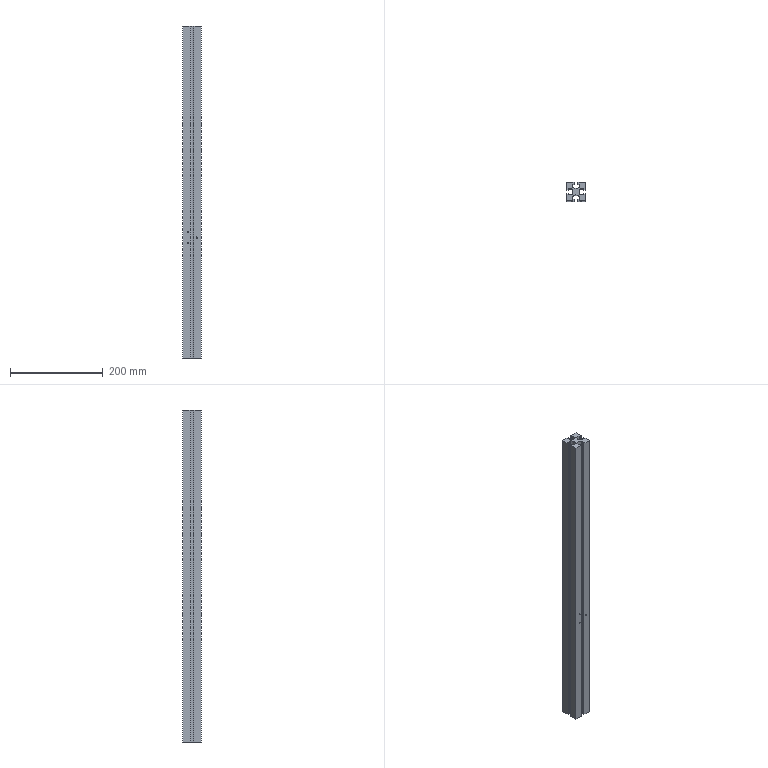Part | NX | 1 solid | 44 faces | box 40 x 40 x 716 mm | volume 715892 mm3 | plane 34 | cylinder 10 | commonest cylinder face diameters 2.5 x6 19.333 x2 19.4 x2
STEP:
#1=CARTESIAN_POINT('',(-125.,655.75,0.));
#2=VERTEX_POINT('',#1);
#3=CARTESIAN_POINT('',(-121.5,655.75,0.));
#4=VERTEX_POINT('',#3);
#5=CARTESIAN_POINT('',(-125.,655.75,0.));
#6=DIRECTION('',(1.,0.,0.));
#7=VECTOR('',#6,1000.);
#8=LINE('',#5,#7);
#9=EDGE_CURVE('',#2,#4,#8,.T.);
#10=ORIENTED_EDGE('',*,*,#9,.T.);
#11=CARTESIAN_POINT('',(-121.5,655.75,-716.));
#12=VERTEX_POINT('',#11);
#13=CARTESIAN_POINT('',(-121.5,655.75,-716.));
#14=DIRECTION('',(0.,0.,1.));
#15=VECTOR('',#14,1000.);
#16=LINE('',#13,#15);
#17=EDGE_CURVE('',#12,#4,#16,.T.);
#18=ORIENTED_EDGE('',*,*,#17,.F.);
#19=CARTESIAN_POINT('',(-125.,655.75,-716.));
#20=VERTEX_POINT('',#19);
#21=CARTESIAN_POINT('',(-125.,655.75,-716.));
#22=DIRECTION('',(1.,0.,0.));
#23=VECTOR('',#22,1000.);
#24=LINE('',#21,#23);
#25=EDGE_CURVE('',#20,#12,#24,.T.);
#26=ORIENTED_EDGE('',*,*,#25,.F.);
#27=CARTESIAN_POINT('',(-125.,655.75,-716.));
#28=DIRECTION('',(0.,0.,1.));
#29=VECTOR('',#28,1000.);
#30=LINE('',#27,#29);
#31=EDGE_CURVE('',#20,#2,#30,.T.);
#32=ORIENTED_EDGE('',*,*,#31,.T.);
#33=EDGE_LOOP('',(#10,#18,#26,#32));
#34=FACE_BOUND('',#33,.T.);
#35=CARTESIAN_POINT('',(-125.,655.75,-716.));
#36=DIRECTION('',(0.,-1.,0.));
#37=DIRECTION('',(0.,0.,-1.));
#38=AXIS2_PLACEMENT_3D('',#35,#36,#37);
#39=PLANE('',#38);
#40=ADVANCED_FACE('',(#34),#39,.F.);
#41=CARTESIAN_POINT('',(-121.5,653.,0.));
#42=VERTEX_POINT('',#41);
#43=CARTESIAN_POINT('',(-121.5,655.75,0.));
#44=DIRECTION('',(0.,-1.,0.));
#45=VECTOR('',#44,1000.);
#46=LINE('',#43,#45);
#47=EDGE_CURVE('',#4,#42,#46,.T.);
#48=ORIENTED_EDGE('',*,*,#47,.T.);
#49=CARTESIAN_POINT('',(-121.5,653.,-716.));
#50=VERTEX_POINT('',#49);
#51=CARTESIAN_POINT('',(-121.5,653.,-716.));
#52=DIRECTION('',(0.,0.,1.));
#53=VECTOR('',#52,1000.);
#54=LINE('',#51,#53);
#55=EDGE_CURVE('',#50,#42,#54,.T.);
#56=ORIENTED_EDGE('',*,*,#55,.F.);
#57=CARTESIAN_POINT('',(-121.5,655.75,-716.));
#58=DIRECTION('',(0.,-1.,0.));
#59=VECTOR('',#58,1000.);
#60=LINE('',#57,#59);
#61=EDGE_CURVE('',#12,#50,#60,.T.);
#62=ORIENTED_EDGE('',*,*,#61,.F.);
#63=ORIENTED_EDGE('',*,*,#17,.T.);
#64=EDGE_LOOP('',(#48,#56,#62,#63));
#65=FACE_BOUND('',#64,.T.);
#66=CARTESIAN_POINT('',(-121.5,655.75,-716.));
#67=DIRECTION('',(-1.,0.,0.));
#68=DIRECTION('',(0.,0.,1.));
#69=AXIS2_PLACEMENT_3D('',#66,#67,#68);
#70=PLANE('',#69);
#71=ADVANCED_FACE('',(#65),#70,.F.);
#72=CARTESIAN_POINT('',(-114.5,653.,-443.965));
#73=VERTEX_POINT('',#72);
#74=CARTESIAN_POINT('',(-114.5,653.,0.));
#75=VERTEX_POINT('',#74);
#76=CARTESIAN_POINT('',(-114.5,653.,-716.));
#77=DIRECTION('',(0.,0.,1.));
#78=VECTOR('',#77,1000.);
#79=LINE('',#76,#78);
#80=EDGE_CURVE('',#73,#75,#79,.T.);
#81=ORIENTED_EDGE('',*,*,#80,.F.);
#82=CARTESIAN_POINT('',(-114.5,653.,-446.205));
#83=VERTEX_POINT('',#82);
#84=CARTESIAN_POINT('',(-113.944,653.,-445.085));
#85=DIRECTION('',(0.,-1.,0.));
#86=DIRECTION('',(0.,0.,-1.));
#87=AXIS2_PLACEMENT_3D('',#84,#85,#86);
#88=CIRCLE('',#87,1.25);
#89=EDGE_CURVE('',#73,#83,#88,.T.);
#90=ORIENTED_EDGE('',*,*,#89,.T.);
#91=CARTESIAN_POINT('',(-114.5,653.,-466.526));
#92=VERTEX_POINT('',#91);
#93=CARTESIAN_POINT('',(-114.5,653.,-716.));
#94=DIRECTION('',(0.,0.,1.));
#95=VECTOR('',#94,1000.);
#96=LINE('',#93,#95);
#97=EDGE_CURVE('',#92,#83,#96,.T.);
#98=ORIENTED_EDGE('',*,*,#97,.F.);
#99=CARTESIAN_POINT('',(-114.5,653.,-468.677));
#100=VERTEX_POINT('',#99);
#101=CARTESIAN_POINT('',(-113.863,653.,-467.601));
#102=DIRECTION('',(0.,-1.,0.));
#103=DIRECTION('',(0.,0.,-1.));
#104=AXIS2_PLACEMENT_3D('',#101,#102,#103);
#105=CIRCLE('',#104,1.25);
#106=EDGE_CURVE('',#92,#100,#105,.T.);
#107=ORIENTED_EDGE('',*,*,#106,.T.);
#108=CARTESIAN_POINT('',(-114.5,653.,-716.));
#109=VERTEX_POINT('',#108);
#110=CARTESIAN_POINT('',(-114.5,653.,-716.));
#111=DIRECTION('',(0.,0.,1.));
#112=VECTOR('',#111,1000.);
#113=LINE('',#110,#112);
#114=EDGE_CURVE('',#109,#100,#113,.T.);
#115=ORIENTED_EDGE('',*,*,#114,.F.);
#116=CARTESIAN_POINT('',(-121.5,653.,-716.));
#117=DIRECTION('',(1.,0.,0.));
#118=VECTOR('',#117,1000.);
#119=LINE('',#116,#118);
#120=EDGE_CURVE('',#50,#109,#119,.T.);
#121=ORIENTED_EDGE('',*,*,#120,.F.);
#122=ORIENTED_EDGE('',*,*,#55,.T.);
#123=CARTESIAN_POINT('',(-121.5,653.,0.));
#124=DIRECTION('',(1.,0.,0.));
#125=VECTOR('',#124,1000.);
#126=LINE('',#123,#125);
#127=EDGE_CURVE('',#42,#75,#126,.T.);
#128=ORIENTED_EDGE('',*,*,#127,.T.);
#129=EDGE_LOOP('',(#81,#90,#98,#107,#115,#121,#122,#128));
#130=FACE_BOUND('',#129,.T.);
#131=CARTESIAN_POINT('',(-121.5,653.,-716.));
#132=DIRECTION('',(0.,-1.,0.));
#133=DIRECTION('',(0.,0.,-1.));
#134=AXIS2_PLACEMENT_3D('',#131,#132,#133);
#135=PLANE('',#134);
#136=ADVANCED_FACE('',(#130),#135,.F.);
#137=ORIENTED_EDGE('',*,*,#97,.T.);
#138=CARTESIAN_POINT('',(-114.5,653.,-446.205));
#139=CARTESIAN_POINT('',(-114.298,653.192,-446.305));
#140=CARTESIAN_POINT('',(-113.888,653.617,-446.38));
#141=CARTESIAN_POINT('',(-113.343,654.301,-446.22));
#142=CARTESIAN_POINT('',(-112.903,654.965,-445.885));
#143=CARTESIAN_POINT('',(-112.59,655.536,-445.087));
#144=CARTESIAN_POINT('',(-112.901,654.969,-444.287));
#145=CARTESIAN_POINT('',(-113.343,654.301,-443.95));
#146=CARTESIAN_POINT('',(-113.889,653.617,-443.79));
#147=CARTESIAN_POINT('',(-114.298,653.192,-443.865));
#148=CARTESIAN_POINT('',(-114.5,653.,-443.965));
#149=B_SPLINE_CURVE_WITH_KNOTS('',3,(#138,#139,#140,#141,#142,#143,#144,#145,#146,#147,#148),.UNSPECIFIED.,.F.,.F.,(4,1,1,1,1,1,1,1,4),(0.,0.0008784,0.001757,0.002635,0.003514,0.004392,0.00527,0.006149,0.007027),.UNSPECIFIED.);
#150=EDGE_CURVE('',#83,#73,#149,.T.);
#151=ORIENTED_EDGE('',*,*,#150,.T.);
#152=ORIENTED_EDGE('',*,*,#80,.T.);
#153=CARTESIAN_POINT('',(-114.5,667.,0.));
#154=VERTEX_POINT('',#153);
#155=CARTESIAN_POINT('',(-121.167,660.,0.));
#156=DIRECTION('',(0.,0.,1.));
#157=DIRECTION('',(-1.,0.,0.));
#158=AXIS2_PLACEMENT_3D('',#155,#156,#157);
#159=CIRCLE('',#158,9.667);
#160=EDGE_CURVE('',#75,#154,#159,.T.);
#161=ORIENTED_EDGE('',*,*,#160,.T.);
#162=CARTESIAN_POINT('',(-114.5,667.,-443.965));
#163=VERTEX_POINT('',#162);
#164=CARTESIAN_POINT('',(-114.5,667.,-716.));
#165=DIRECTION('',(0.,0.,1.));
#166=VECTOR('',#165,1000.);
#167=LINE('',#164,#166);
#168=EDGE_CURVE('',#163,#154,#167,.T.);
#169=ORIENTED_EDGE('',*,*,#168,.F.);
#170=CARTESIAN_POINT('',(-114.5,667.,-446.205));
#171=VERTEX_POINT('',#170);
#172=CARTESIAN_POINT('',(-114.5,667.,-443.965));
#173=CARTESIAN_POINT('',(-114.298,666.808,-443.865));
#174=CARTESIAN_POINT('',(-113.888,666.383,-443.79));
#175=CARTESIAN_POINT('',(-113.343,665.699,-443.95));
#176=CARTESIAN_POINT('',(-112.903,665.035,-444.285));
#177=CARTESIAN_POINT('',(-112.59,664.464,-445.083));
#178=CARTESIAN_POINT('',(-112.901,665.031,-445.883));
#179=CARTESIAN_POINT('',(-113.343,665.699,-446.22));
#180=CARTESIAN_POINT('',(-113.889,666.383,-446.379));
#181=CARTESIAN_POINT('',(-114.298,666.808,-446.305));
#182=CARTESIAN_POINT('',(-114.5,667.,-446.205));
#183=B_SPLINE_CURVE_WITH_KNOTS('',3,(#172,#173,#174,#175,#176,#177,#178,#179,#180,#181,#182),.UNSPECIFIED.,.F.,.F.,(4,1,1,1,1,1,1,1,4),(0.,0.0008784,0.001757,0.002635,0.003514,0.004392,0.00527,0.006149,0.007027),.UNSPECIFIED.);
#184=EDGE_CURVE('',#163,#171,#183,.T.);
#185=ORIENTED_EDGE('',*,*,#184,.T.);
#186=CARTESIAN_POINT('',(-114.5,667.,-466.526));
#187=VERTEX_POINT('',#186);
#188=CARTESIAN_POINT('',(-114.5,667.,-716.));
#189=DIRECTION('',(0.,0.,1.));
#190=VECTOR('',#189,1000.);
#191=LINE('',#188,#190);
#192=EDGE_CURVE('',#187,#171,#191,.T.);
#193=ORIENTED_EDGE('',*,*,#192,.F.);
#194=CARTESIAN_POINT('',(-114.5,667.,-468.677));
#195=VERTEX_POINT('',#194);
#196=CARTESIAN_POINT('',(-114.5,667.,-466.526));
#197=CARTESIAN_POINT('',(-114.293,666.803,-466.403));
#198=CARTESIAN_POINT('',(-113.865,666.357,-466.304));
#199=CARTESIAN_POINT('',(-113.295,665.635,-466.44));
#200=CARTESIAN_POINT('',(-112.908,665.035,-466.748));
#201=CARTESIAN_POINT('',(-112.674,664.621,-467.149));
#202=CARTESIAN_POINT('',(-112.582,664.443,-467.602));
#203=CARTESIAN_POINT('',(-112.675,664.622,-468.056));
#204=CARTESIAN_POINT('',(-112.909,665.037,-468.456));
#205=CARTESIAN_POINT('',(-113.296,665.637,-468.763));
#206=CARTESIAN_POINT('',(-113.864,666.357,-468.899));
#207=CARTESIAN_POINT('',(-114.293,666.803,-468.799));
#208=CARTESIAN_POINT('',(-114.5,667.,-468.677));
#209=B_SPLINE_CURVE_WITH_KNOTS('',3,(#196,#197,#198,#199,#200,#201,#202,#203,#204,#205,#206,#207,#208),.UNSPECIFIED.,.F.,.F.,(4,1,1,1,1,1,1,1,1,1,4),(0.,0.0009217,0.001843,0.002765,0.003226,0.003687,0.004148,0.004608,0.00553,0.006452,0.007373),.UNSPECIFIED.);
#210=EDGE_CURVE('',#187,#195,#209,.T.);
#211=ORIENTED_EDGE('',*,*,#210,.T.);
#212=CARTESIAN_POINT('',(-114.5,667.,-716.));
#213=VERTEX_POINT('',#212);
#214=CARTESIAN_POINT('',(-114.5,667.,-716.));
#215=DIRECTION('',(0.,0.,1.));
#216=VECTOR('',#215,1000.);
#217=LINE('',#214,#216);
#218=EDGE_CURVE('',#213,#195,#217,.T.);
#219=ORIENTED_EDGE('',*,*,#218,.F.);
#220=CARTESIAN_POINT('',(-121.167,660.,-716.));
#221=DIRECTION('',(0.,0.,1.));
#222=DIRECTION('',(-1.,0.,0.));
#223=AXIS2_PLACEMENT_3D('',#220,#221,#222);
#224=CIRCLE('',#223,9.667);
#225=EDGE_CURVE('',#109,#213,#224,.T.);
#226=ORIENTED_EDGE('',*,*,#225,.F.);
#227=ORIENTED_EDGE('',*,*,#114,.T.);
#228=CARTESIAN_POINT('',(-114.5,653.,-468.677));
#229=CARTESIAN_POINT('',(-114.293,653.197,-468.799));
#230=CARTESIAN_POINT('',(-113.865,653.643,-468.899));
#231=CARTESIAN_POINT('',(-113.295,654.365,-468.763));
#232=CARTESIAN_POINT('',(-112.908,654.965,-468.455));
#233=CARTESIAN_POINT('',(-112.674,655.379,-468.054));
#234=CARTESIAN_POINT('',(-112.582,655.557,-467.6));
#235=CARTESIAN_POINT('',(-112.675,655.378,-467.147));
#236=CARTESIAN_POINT('',(-112.909,654.963,-466.747));
#237=CARTESIAN_POINT('',(-113.296,654.363,-466.44));
#238=CARTESIAN_POINT('',(-113.864,653.643,-466.304));
#239=CARTESIAN_POINT('',(-114.293,653.197,-466.404));
#240=CARTESIAN_POINT('',(-114.5,653.,-466.526));
#241=B_SPLINE_CURVE_WITH_KNOTS('',3,(#228,#229,#230,#231,#232,#233,#234,#235,#236,#237,#238,#239,#240),.UNSPECIFIED.,.F.,.F.,(4,1,1,1,1,1,1,1,1,1,4),(0.,0.0009217,0.001843,0.002765,0.003226,0.003687,0.004148,0.004608,0.00553,0.006452,0.007373),.UNSPECIFIED.);
#242=EDGE_CURVE('',#100,#92,#241,.T.);
#243=ORIENTED_EDGE('',*,*,#242,.T.);
#244=EDGE_LOOP('',(#137,#151,#152,#161,#169,#185,#193,#211,#219,#226,#227,#243));
#245=FACE_BOUND('',#244,.T.);
#246=CARTESIAN_POINT('',(-121.167,660.,-716.));
#247=DIRECTION('',(0.,0.,1.));
#248=DIRECTION('',(1.,0.,0.));
#249=AXIS2_PLACEMENT_3D('',#246,#247,#248);
#250=CYLINDRICAL_SURFACE('',#249,9.667);
#251=ADVANCED_FACE('',(#245),#250,.F.);
#252=ORIENTED_EDGE('',*,*,#192,.T.);
#253=CARTESIAN_POINT('',(-113.944,667.,-445.085));
#254=DIRECTION('',(0.,1.,0.));
#255=DIRECTION('',(0.,0.,1.));
#256=AXIS2_PLACEMENT_3D('',#253,#254,#255);
#257=CIRCLE('',#256,1.25);
#258=EDGE_CURVE('',#171,#163,#257,.T.);
#259=ORIENTED_EDGE('',*,*,#258,.T.);
#260=ORIENTED_EDGE('',*,*,#168,.T.);
#261=CARTESIAN_POINT('',(-121.5,667.,0.));
#262=VERTEX_POINT('',#261);
#263=CARTESIAN_POINT('',(-114.5,667.,0.));
#264=DIRECTION('',(-1.,0.,0.));
#265=VECTOR('',#264,1000.);
#266=LINE('',#263,#265);
#267=EDGE_CURVE('',#154,#262,#266,.T.);
#268=ORIENTED_EDGE('',*,*,#267,.T.);
#269=CARTESIAN_POINT('',(-121.5,667.,-716.));
#270=VERTEX_POINT('',#269);
#271=CARTESIAN_POINT('',(-121.5,667.,-716.));
#272=DIRECTION('',(0.,0.,1.));
#273=VECTOR('',#272,1000.);
#274=LINE('',#271,#273);
#275=EDGE_CURVE('',#270,#262,#274,.T.);
#276=ORIENTED_EDGE('',*,*,#275,.F.);
#277=CARTESIAN_POINT('',(-114.5,667.,-716.));
#278=DIRECTION('',(-1.,0.,0.));
#279=VECTOR('',#278,1000.);
#280=LINE('',#277,#279);
#281=EDGE_CURVE('',#213,#270,#280,.T.);
#282=ORIENTED_EDGE('',*,*,#281,.F.);
#283=ORIENTED_EDGE('',*,*,#218,.T.);
#284=CARTESIAN_POINT('',(-113.863,667.,-467.601));
#285=DIRECTION('',(0.,1.,0.));
#286=DIRECTION('',(0.,0.,1.));
#287=AXIS2_PLACEMENT_3D('',#284,#285,#286);
#288=CIRCLE('',#287,1.25);
#289=EDGE_CURVE('',#195,#187,#288,.T.);
#290=ORIENTED_EDGE('',*,*,#289,.T.);
#291=EDGE_LOOP('',(#252,#259,#260,#268,#276,#282,#283,#290));
#292=FACE_BOUND('',#291,.T.);
#293=CARTESIAN_POINT('',(-114.5,667.,-716.));
#294=DIRECTION('',(0.,1.,0.));
#295=DIRECTION('',(0.,0.,1.));
#296=AXIS2_PLACEMENT_3D('',#293,#294,#295);
#297=PLANE('',#296);
#298=ADVANCED_FACE('',(#292),#297,.F.);
#299=CARTESIAN_POINT('',(-121.5,664.25,0.));
#300=VERTEX_POINT('',#299);
#301=CARTESIAN_POINT('',(-121.5,667.,0.));
#302=DIRECTION('',(0.,-1.,0.));
#303=VECTOR('',#302,1000.);
#304=LINE('',#301,#303);
#305=EDGE_CURVE('',#262,#300,#304,.T.);
#306=ORIENTED_EDGE('',*,*,#305,.T.);
#307=CARTESIAN_POINT('',(-121.5,664.25,-716.));
#308=VERTEX_POINT('',#307);
#309=CARTESIAN_POINT('',(-121.5,664.25,-716.));
#310=DIRECTION('',(0.,0.,1.));
#311=VECTOR('',#310,1000.);
#312=LINE('',#309,#311);
#313=EDGE_CURVE('',#308,#300,#312,.T.);
#314=ORIENTED_EDGE('',*,*,#313,.F.);
#315=CARTESIAN_POINT('',(-121.5,667.,-716.));
#316=DIRECTION('',(0.,-1.,0.));
#317=VECTOR('',#316,1000.);
#318=LINE('',#315,#317);
#319=EDGE_CURVE('',#270,#308,#318,.T.);
#320=ORIENTED_EDGE('',*,*,#319,.F.);
#321=ORIENTED_EDGE('',*,*,#275,.T.);
#322=EDGE_LOOP('',(#306,#314,#320,#321));
#323=FACE_BOUND('',#322,.T.);
#324=CARTESIAN_POINT('',(-121.5,667.,-716.));
#325=DIRECTION('',(-1.,0.,0.));
#326=DIRECTION('',(0.,0.,1.));
#327=AXIS2_PLACEMENT_3D('',#324,#325,#326);
#328=PLANE('',#327);
#329=ADVANCED_FACE('',(#323),#328,.F.);
#330=CARTESIAN_POINT('',(-125.,664.25,0.));
#331=VERTEX_POINT('',#330);
#332=CARTESIAN_POINT('',(-121.5,664.25,0.));
#333=DIRECTION('',(-1.,0.,0.));
#334=VECTOR('',#333,1000.);
#335=LINE('',#332,#334);
#336=EDGE_CURVE('',#300,#331,#335,.T.);
#337=ORIENTED_EDGE('',*,*,#336,.T.);
#338=CARTESIAN_POINT('',(-125.,664.25,-716.));
#339=VERTEX_POINT('',#338);
#340=CARTESIAN_POINT('',(-125.,664.25,-716.));
#341=DIRECTION('',(0.,0.,1.));
#342=VECTOR('',#341,1000.);
#343=LINE('',#340,#342);
#344=EDGE_CURVE('',#339,#331,#343,.T.);
#345=ORIENTED_EDGE('',*,*,#344,.F.);
#346=CARTESIAN_POINT('',(-121.5,664.25,-716.));
#347=DIRECTION('',(-1.,0.,0.));
#348=VECTOR('',#347,1000.);
#349=LINE('',#346,#348);
#350=EDGE_CURVE('',#308,#339,#349,.T.);
#351=ORIENTED_EDGE('',*,*,#350,.F.);
#352=ORIENTED_EDGE('',*,*,#313,.T.);
#353=EDGE_LOOP('',(#337,#345,#351,#352));
#354=FACE_BOUND('',#353,.T.);
#355=CARTESIAN_POINT('',(-121.5,664.25,-716.));
#356=DIRECTION('',(0.,1.,0.));
#357=DIRECTION('',(0.,0.,1.));
#358=AXIS2_PLACEMENT_3D('',#355,#356,#357);
#359=PLANE('',#358);
#360=ADVANCED_FACE('',(#354),#359,.F.);
#361=CARTESIAN_POINT('',(-125.,680.,0.));
#362=VERTEX_POINT('',#361);
#363=CARTESIAN_POINT('',(-125.,680.,0.));
#364=DIRECTION('',(0.,1.,0.));
#365=VECTOR('',#364,1000.);
#366=LINE('',#363,#365);
#367=EDGE_CURVE('',#331,#362,#366,.T.);
#368=ORIENTED_EDGE('',*,*,#367,.T.);
#369=CARTESIAN_POINT('',(-125.,680.,-716.));
#370=VERTEX_POINT('',#369);
#371=CARTESIAN_POINT('',(-125.,680.,-716.));
#372=DIRECTION('',(0.,0.,1.));
#373=VECTOR('',#372,1000.);
#374=LINE('',#371,#373);
#375=EDGE_CURVE('',#370,#362,#374,.T.);
#376=ORIENTED_EDGE('',*,*,#375,.F.);
#377=CARTESIAN_POINT('',(-125.,664.25,-716.));
#378=DIRECTION('',(0.,1.,0.));
#379=VECTOR('',#378,1000.);
#380=LINE('',#377,#379);
#381=EDGE_CURVE('',#339,#370,#380,.T.);
#382=ORIENTED_EDGE('',*,*,#381,.F.);
#383=ORIENTED_EDGE('',*,*,#344,.T.);
#384=EDGE_LOOP('',(#368,#376,#382,#383));
#385=FACE_BOUND('',#384,.T.);
#386=CARTESIAN_POINT('',(-125.,680.,-716.));
#387=DIRECTION('',(1.,0.,0.));
#388=DIRECTION('',(0.,0.,-1.));
#389=AXIS2_PLACEMENT_3D('',#386,#387,#388);
#390=PLANE('',#389);
#391=ADVANCED_FACE('',(#385),#390,.F.);
#392=CARTESIAN_POINT('',(-113.944,680.,-443.835));
#393=VERTEX_POINT('',#392);
#394=CARTESIAN_POINT('',(-113.944,680.,-445.085));
#395=DIRECTION('',(0.,1.,0.));
#396=DIRECTION('',(0.,0.,1.));
#397=AXIS2_PLACEMENT_3D('',#394,#395,#396);
#398=CIRCLE('',#397,1.25);
#399=EDGE_CURVE('',#393,#393,#398,.T.);
#400=ORIENTED_EDGE('',*,*,#399,.F.);
#401=EDGE_LOOP('',(#400));
#402=FACE_BOUND('',#401,.T.);
#403=CARTESIAN_POINT('',(-113.863,680.,-466.351));
#404=VERTEX_POINT('',#403);
#405=CARTESIAN_POINT('',(-113.863,680.,-467.601));
#406=DIRECTION('',(0.,1.,0.));
#407=DIRECTION('',(0.,0.,1.));
#408=AXIS2_PLACEMENT_3D('',#405,#406,#407);
#409=CIRCLE('',#408,1.25);
#410=EDGE_CURVE('',#404,#404,#409,.T.);
#411=ORIENTED_EDGE('',*,*,#410,.F.);
#412=EDGE_LOOP('',(#411));
#413=FACE_BOUND('',#412,.T.);
#414=CARTESIAN_POINT('',(-109.25,680.,0.));
#415=VERTEX_POINT('',#414);
#416=CARTESIAN_POINT('',(-124.5,680.,0.));
#417=DIRECTION('',(1.,0.,0.));
#418=VECTOR('',#417,1000.);
#419=LINE('',#416,#418);
#420=EDGE_CURVE('',#362,#415,#419,.T.);
#421=ORIENTED_EDGE('',*,*,#420,.T.);
#422=CARTESIAN_POINT('',(-109.25,680.,-716.));
#423=VERTEX_POINT('',#422);
#424=CARTESIAN_POINT('',(-109.25,680.,-716.));
#425=DIRECTION('',(0.,0.,1.));
#426=VECTOR('',#425,1000.);
#427=LINE('',#424,#426);
#428=EDGE_CURVE('',#423,#415,#427,.T.);
#429=ORIENTED_EDGE('',*,*,#428,.F.);
#430=CARTESIAN_POINT('',(-124.5,680.,-716.));
#431=DIRECTION('',(1.,0.,0.));
#432=VECTOR('',#431,1000.);
#433=LINE('',#430,#432);
#434=EDGE_CURVE('',#370,#423,#433,.T.);
#435=ORIENTED_EDGE('',*,*,#434,.F.);
#436=ORIENTED_EDGE('',*,*,#375,.T.);
#437=EDGE_LOOP('',(#421,#429,#435,#436));
#438=FACE_BOUND('',#437,.T.);
#439=CARTESIAN_POINT('',(-124.5,680.,-716.));
#440=DIRECTION('',(0.,-1.,0.));
#441=DIRECTION('',(0.,0.,-1.));
#442=AXIS2_PLACEMENT_3D('',#439,#440,#441);
#443=PLANE('',#442);
#444=ADVANCED_FACE('',(#402,#413,#438),#443,.F.);
#445=CARTESIAN_POINT('',(-109.25,676.5,0.));
#446=VERTEX_POINT('',#445);
#447=CARTESIAN_POINT('',(-109.25,680.,0.));
#448=DIRECTION('',(0.,-1.,0.));
#449=VECTOR('',#448,1000.);
#450=LINE('',#447,#449);
#451=EDGE_CURVE('',#415,#446,#450,.T.);
#452=ORIENTED_EDGE('',*,*,#451,.T.);
#453=CARTESIAN_POINT('',(-109.25,676.5,-716.));
#454=VERTEX_POINT('',#453);
#455=CARTESIAN_POINT('',(-109.25,676.5,-716.));
#456=DIRECTION('',(0.,0.,1.));
#457=VECTOR('',#456,1000.);
#458=LINE('',#455,#457);
#459=EDGE_CURVE('',#454,#446,#458,.T.);
#460=ORIENTED_EDGE('',*,*,#459,.F.);
#461=CARTESIAN_POINT('',(-109.25,680.,-716.));
#462=DIRECTION('',(0.,-1.,0.));
#463=VECTOR('',#462,1000.);
#464=LINE('',#461,#463);
#465=EDGE_CURVE('',#423,#454,#464,.T.);
#466=ORIENTED_EDGE('',*,*,#465,.F.);
#467=ORIENTED_EDGE('',*,*,#428,.T.);
#468=EDGE_LOOP('',(#452,#460,#466,#467));
#469=FACE_BOUND('',#468,.T.);
#470=CARTESIAN_POINT('',(-109.25,680.,-716.));
#471=DIRECTION('',(-1.,0.,0.));
#472=DIRECTION('',(0.,0.,1.));
#473=AXIS2_PLACEMENT_3D('',#470,#471,#472);
#474=PLANE('',#473);
#475=ADVANCED_FACE('',(#469),#474,.F.);
#476=CARTESIAN_POINT('',(-111.5,676.5,0.));
#477=VERTEX_POINT('',#476);
#478=CARTESIAN_POINT('',(-109.25,676.5,0.));
#479=DIRECTION('',(-1.,0.,0.));
#480=VECTOR('',#479,1000.);
#481=LINE('',#478,#480);
#482=EDGE_CURVE('',#446,#477,#481,.T.);
#483=ORIENTED_EDGE('',*,*,#482,.T.);
#484=CARTESIAN_POINT('',(-111.5,676.5,-716.));
#485=VERTEX_POINT('',#484);
#486=CARTESIAN_POINT('',(-111.5,676.5,-716.));
#487=DIRECTION('',(0.,0.,1.));
#488=VECTOR('',#487,1000.);
#489=LINE('',#486,#488);
#490=EDGE_CURVE('',#485,#477,#489,.T.);
#491=ORIENTED_EDGE('',*,*,#490,.F.);
#492=CARTESIAN_POINT('',(-109.25,676.5,-716.));
#493=DIRECTION('',(-1.,0.,0.));
#494=VECTOR('',#493,1000.);
#495=LINE('',#492,#494);
#496=EDGE_CURVE('',#454,#485,#495,.T.);
#497=ORIENTED_EDGE('',*,*,#496,.F.);
#498=ORIENTED_EDGE('',*,*,#459,.T.);
#499=EDGE_LOOP('',(#483,#491,#497,#498));
#500=FACE_BOUND('',#499,.T.);
#501=CARTESIAN_POINT('',(-109.25,676.5,-716.));
#502=DIRECTION('',(0.,1.,0.));
#503=DIRECTION('',(0.,0.,1.));
#504=AXIS2_PLACEMENT_3D('',#501,#502,#503);
#505=PLANE('',#504);
#506=ADVANCED_FACE('',(#500),#505,.F.);
#507=CARTESIAN_POINT('',(-111.5,669.5,0.));
#508=VERTEX_POINT('',#507);
#509=CARTESIAN_POINT('',(-111.5,676.5,0.));
#510=DIRECTION('',(0.,-1.,0.));
#511=VECTOR('',#510,1000.);
#512=LINE('',#509,#511);
#513=EDGE_CURVE('',#477,#508,#512,.T.);
#514=ORIENTED_EDGE('',*,*,#513,.T.);
#515=CARTESIAN_POINT('',(-111.5,669.5,-716.));
#516=VERTEX_POINT('',#515);
#517=CARTESIAN_POINT('',(-111.5,669.5,-716.));
#518=DIRECTION('',(0.,0.,1.));
#519=VECTOR('',#518,1000.);
#520=LINE('',#517,#519);
#521=EDGE_CURVE('',#516,#508,#520,.T.);
#522=ORIENTED_EDGE('',*,*,#521,.F.);
#523=CARTESIAN_POINT('',(-111.5,676.5,-716.));
#524=DIRECTION('',(0.,-1.,0.));
#525=VECTOR('',#524,1000.);
#526=LINE('',#523,#525);
#527=EDGE_CURVE('',#485,#516,#526,.T.);
#528=ORIENTED_EDGE('',*,*,#527,.F.);
#529=ORIENTED_EDGE('',*,*,#490,.T.);
#530=EDGE_LOOP('',(#514,#522,#528,#529));
#531=FACE_BOUND('',#530,.T.);
#532=CARTESIAN_POINT('',(-111.5,676.5,-716.));
#533=DIRECTION('',(-1.,0.,0.));
#534=DIRECTION('',(0.,0.,1.));
#535=AXIS2_PLACEMENT_3D('',#532,#533,#534);
#536=PLANE('',#535);
#537=ADVANCED_FACE('',(#531),#536,.F.);
#538=CARTESIAN_POINT('',(-98.5,669.5,0.));
#539=VERTEX_POINT('',#538);
#540=CARTESIAN_POINT('',(-105.,676.7,0.));
#541=DIRECTION('',(0.,0.,1.));
#542=DIRECTION('',(-1.,0.,0.));
#543=AXIS2_PLACEMENT_3D('',#540,#541,#542);
#544=CIRCLE('',#543,9.7);
#545=EDGE_CURVE('',#508,#539,#544,.T.);
#546=ORIENTED_EDGE('',*,*,#545,.T.);
#547=CARTESIAN_POINT('',(-98.5,669.5,-716.));
#548=VERTEX_POINT('',#547);
#549=CARTESIAN_POINT('',(-98.5,669.5,-716.));
#550=DIRECTION('',(0.,0.,1.));
#551=VECTOR('',#550,1000.);
#552=LINE('',#549,#551);
#553=EDGE_CURVE('',#548,#539,#552,.T.);
#554=ORIENTED_EDGE('',*,*,#553,.F.);
#555=CARTESIAN_POINT('',(-105.,676.7,-716.));
#556=DIRECTION('',(0.,0.,1.));
#557=DIRECTION('',(-1.,0.,0.));
#558=AXIS2_PLACEMENT_3D('',#555,#556,#557);
#559=CIRCLE('',#558,9.7);
#560=EDGE_CURVE('',#516,#548,#559,.T.);
#561=ORIENTED_EDGE('',*,*,#560,.F.);
#562=ORIENTED_EDGE('',*,*,#521,.T.);
#563=EDGE_LOOP('',(#546,#554,#561,#562));
#564=FACE_BOUND('',#563,.T.);
#565=CARTESIAN_POINT('',(-105.,676.7,-716.));
#566=DIRECTION('',(0.,0.,1.));
#567=DIRECTION('',(1.,0.,0.));
#568=AXIS2_PLACEMENT_3D('',#565,#566,#567);
#569=CYLINDRICAL_SURFACE('',#568,9.7);
#570=ADVANCED_FACE('',(#564),#569,.F.);
#571=CARTESIAN_POINT('',(-98.5,676.5,0.));
#572=VERTEX_POINT('',#571);
#573=CARTESIAN_POINT('',(-98.5,669.5,0.));
#574=DIRECTION('',(0.,1.,0.));
#575=VECTOR('',#574,1000.);
#576=LINE('',#573,#575);
#577=EDGE_CURVE('',#539,#572,#576,.T.);
#578=ORIENTED_EDGE('',*,*,#577,.T.);
#579=CARTESIAN_POINT('',(-98.5,676.5,-716.));
#580=VERTEX_POINT('',#579);
#581=CARTESIAN_POINT('',(-98.5,676.5,-716.));
#582=DIRECTION('',(0.,0.,1.));
#583=VECTOR('',#582,1000.);
#584=LINE('',#581,#583);
#585=EDGE_CURVE('',#580,#572,#584,.T.);
#586=ORIENTED_EDGE('',*,*,#585,.F.);
#587=CARTESIAN_POINT('',(-98.5,669.5,-716.));
#588=DIRECTION('',(0.,1.,0.));
#589=VECTOR('',#588,1000.);
#590=LINE('',#587,#589);
#591=EDGE_CURVE('',#548,#580,#590,.T.);
#592=ORIENTED_EDGE('',*,*,#591,.F.);
#593=ORIENTED_EDGE('',*,*,#553,.T.);
#594=EDGE_LOOP('',(#578,#586,#592,#593));
#595=FACE_BOUND('',#594,.T.);
#596=CARTESIAN_POINT('',(-98.5,669.5,-716.));
#597=DIRECTION('',(1.,0.,0.));
#598=DIRECTION('',(0.,0.,-1.));
#599=AXIS2_PLACEMENT_3D('',#596,#597,#598);
#600=PLANE('',#599);
#601=ADVANCED_FACE('',(#595),#600,.F.);
#602=CARTESIAN_POINT('',(-100.75,676.5,0.));
#603=VERTEX_POINT('',#602);
#604=CARTESIAN_POINT('',(-98.5,676.5,0.));
#605=DIRECTION('',(-1.,0.,0.));
#606=VECTOR('',#605,1000.);
#607=LINE('',#604,#606);
#608=EDGE_CURVE('',#572,#603,#607,.T.);
#609=ORIENTED_EDGE('',*,*,#608,.T.);
#610=CARTESIAN_POINT('',(-100.75,676.5,-716.));
#611=VERTEX_POINT('',#610);
#612=CARTESIAN_POINT('',(-100.75,676.5,-716.));
#613=DIRECTION('',(0.,0.,1.));
#614=VECTOR('',#613,1000.);
#615=LINE('',#612,#614);
#616=EDGE_CURVE('',#611,#603,#615,.T.);
#617=ORIENTED_EDGE('',*,*,#616,.F.);
#618=CARTESIAN_POINT('',(-98.5,676.5,-716.));
#619=DIRECTION('',(-1.,0.,0.));
#620=VECTOR('',#619,1000.);
#621=LINE('',#618,#620);
#622=EDGE_CURVE('',#580,#611,#621,.T.);
#623=ORIENTED_EDGE('',*,*,#622,.F.);
#624=ORIENTED_EDGE('',*,*,#585,.T.);
#625=EDGE_LOOP('',(#609,#617,#623,#624));
#626=FACE_BOUND('',#625,.T.);
#627=CARTESIAN_POINT('',(-98.5,676.5,-716.));
#628=DIRECTION('',(0.,1.,0.));
#629=DIRECTION('',(0.,0.,1.));
#630=AXIS2_PLACEMENT_3D('',#627,#628,#629);
#631=PLANE('',#630);
#632=ADVANCED_FACE('',(#626),#631,.F.);
#633=CARTESIAN_POINT('',(-100.75,680.,0.));
#634=VERTEX_POINT('',#633);
#635=CARTESIAN_POINT('',(-100.75,676.5,0.));
#636=DIRECTION('',(0.,1.,0.));
#637=VECTOR('',#636,1000.);
#638=LINE('',#635,#637);
#639=EDGE_CURVE('',#603,#634,#638,.T.);
#640=ORIENTED_EDGE('',*,*,#639,.T.);
#641=CARTESIAN_POINT('',(-100.75,680.,-716.));
#642=VERTEX_POINT('',#641);
#643=CARTESIAN_POINT('',(-100.75,680.,-716.));
#644=DIRECTION('',(0.,0.,1.));
#645=VECTOR('',#644,1000.);
#646=LINE('',#643,#645);
#647=EDGE_CURVE('',#642,#634,#646,.T.);
#648=ORIENTED_EDGE('',*,*,#647,.F.);
#649=CARTESIAN_POINT('',(-100.75,676.5,-716.));
#650=DIRECTION('',(0.,1.,0.));
#651=VECTOR('',#650,1000.);
#652=LINE('',#649,#651);
#653=EDGE_CURVE('',#611,#642,#652,.T.);
#654=ORIENTED_EDGE('',*,*,#653,.F.);
#655=ORIENTED_EDGE('',*,*,#616,.T.);
#656=EDGE_LOOP('',(#640,#648,#654,#655));
#657=FACE_BOUND('',#656,.T.);
#658=CARTESIAN_POINT('',(-100.75,676.5,-716.));
#659=DIRECTION('',(1.,0.,0.));
#660=DIRECTION('',(0.,0.,-1.));
#661=AXIS2_PLACEMENT_3D('',#658,#659,#660);
#662=PLANE('',#661);
#663=ADVANCED_FACE('',(#657),#662,.F.);
#664=CARTESIAN_POINT('',(-94.403,680.,-455.023));
#665=VERTEX_POINT('',#664);
#666=CARTESIAN_POINT('',(-94.403,680.,-456.273));
#667=DIRECTION('',(0.,1.,0.));
#668=DIRECTION('',(0.,0.,1.));
#669=AXIS2_PLACEMENT_3D('',#666,#667,#668);
#670=CIRCLE('',#669,1.25);
#671=EDGE_CURVE('',#665,#665,#670,.T.);
#672=ORIENTED_EDGE('',*,*,#671,.F.);
#673=EDGE_LOOP('',(#672));
#674=FACE_BOUND('',#673,.T.);
#675=CARTESIAN_POINT('',(-85.,680.,0.));
#676=VERTEX_POINT('',#675);
#677=CARTESIAN_POINT('',(-85.5,680.,0.));
#678=DIRECTION('',(1.,0.,0.));
#679=VECTOR('',#678,1000.);
#680=LINE('',#677,#679);
#681=EDGE_CURVE('',#634,#676,#680,.T.);
#682=ORIENTED_EDGE('',*,*,#681,.T.);
#683=CARTESIAN_POINT('',(-85.,680.,-716.));
#684=VERTEX_POINT('',#683);
#685=CARTESIAN_POINT('',(-85.,680.,-716.));
#686=DIRECTION('',(0.,0.,1.));
#687=VECTOR('',#686,1000.);
#688=LINE('',#685,#687);
#689=EDGE_CURVE('',#684,#676,#688,.T.);
#690=ORIENTED_EDGE('',*,*,#689,.F.);
#691=CARTESIAN_POINT('',(-100.75,680.,-716.));
#692=DIRECTION('',(1.,0.,0.));
#693=VECTOR('',#692,1000.);
#694=LINE('',#691,#693);
#695=EDGE_CURVE('',#642,#684,#694,.T.);
#696=ORIENTED_EDGE('',*,*,#695,.F.);
#697=ORIENTED_EDGE('',*,*,#647,.T.);
#698=EDGE_LOOP('',(#682,#690,#696,#697));
#699=FACE_BOUND('',#698,.T.);
#700=CARTESIAN_POINT('',(-85.5,680.,-716.));
#701=DIRECTION('',(0.,-1.,0.));
#702=DIRECTION('',(0.,0.,-1.));
#703=AXIS2_PLACEMENT_3D('',#700,#701,#702);
#704=PLANE('',#703);
#705=ADVANCED_FACE('',(#674,#699),#704,.F.);
#706=CARTESIAN_POINT('',(-85.,664.25,0.));
#707=VERTEX_POINT('',#706);
#708=CARTESIAN_POINT('',(-85.,679.5,0.));
#709=DIRECTION('',(0.,-1.,0.));
#710=VECTOR('',#709,1000.);
#711=LINE('',#708,#710);
#712=EDGE_CURVE('',#676,#707,#711,.T.);
#713=ORIENTED_EDGE('',*,*,#712,.T.);
#714=CARTESIAN_POINT('',(-85.,664.25,-716.));
#715=VERTEX_POINT('',#714);
#716=CARTESIAN_POINT('',(-85.,664.25,-716.));
#717=DIRECTION('',(0.,0.,1.));
#718=VECTOR('',#717,1000.);
#719=LINE('',#716,#718);
#720=EDGE_CURVE('',#715,#707,#719,.T.);
#721=ORIENTED_EDGE('',*,*,#720,.F.);
#722=CARTESIAN_POINT('',(-85.,680.,-716.));
#723=DIRECTION('',(0.,-1.,0.));
#724=VECTOR('',#723,1000.);
#725=LINE('',#722,#724);
#726=EDGE_CURVE('',#684,#715,#725,.T.);
#727=ORIENTED_EDGE('',*,*,#726,.F.);
#728=ORIENTED_EDGE('',*,*,#689,.T.);
#729=EDGE_LOOP('',(#713,#721,#727,#728));
#730=FACE_BOUND('',#729,.T.);
#731=CARTESIAN_POINT('',(-85.,679.5,-716.));
#732=DIRECTION('',(-1.,0.,0.));
#733=DIRECTION('',(0.,0.,1.));
#734=AXIS2_PLACEMENT_3D('',#731,#732,#733);
#735=PLANE('',#734);
#736=ADVANCED_FACE('',(#730),#735,.F.);
#737=CARTESIAN_POINT('',(-88.5,664.25,0.));
#738=VERTEX_POINT('',#737);
#739=CARTESIAN_POINT('',(-85.,664.25,0.));
#740=DIRECTION('',(-1.,0.,0.));
#741=VECTOR('',#740,1000.);
#742=LINE('',#739,#741);
#743=EDGE_CURVE('',#707,#738,#742,.T.);
#744=ORIENTED_EDGE('',*,*,#743,.T.);
#745=CARTESIAN_POINT('',(-88.5,664.25,-716.));
#746=VERTEX_POINT('',#745);
#747=CARTESIAN_POINT('',(-88.5,664.25,-716.));
#748=DIRECTION('',(0.,0.,1.));
#749=VECTOR('',#748,1000.);
#750=LINE('',#747,#749);
#751=EDGE_CURVE('',#746,#738,#750,.T.);
#752=ORIENTED_EDGE('',*,*,#751,.F.);
#753=CARTESIAN_POINT('',(-85.,664.25,-716.));
#754=DIRECTION('',(-1.,0.,0.));
#755=VECTOR('',#754,1000.);
#756=LINE('',#753,#755);
#757=EDGE_CURVE('',#715,#746,#756,.T.);
#758=ORIENTED_EDGE('',*,*,#757,.F.);
#759=ORIENTED_EDGE('',*,*,#720,.T.);
#760=EDGE_LOOP('',(#744,#752,#758,#759));
#761=FACE_BOUND('',#760,.T.);
#762=CARTESIAN_POINT('',(-85.,664.25,-716.));
#763=DIRECTION('',(0.,1.,0.));
#764=DIRECTION('',(0.,0.,1.));
#765=AXIS2_PLACEMENT_3D('',#762,#763,#764);
#766=PLANE('',#765);
#767=ADVANCED_FACE('',(#761),#766,.F.);
#768=CARTESIAN_POINT('',(-88.5,667.,0.));
#769=VERTEX_POINT('',#768);
#770=CARTESIAN_POINT('',(-88.5,664.25,0.));
#771=DIRECTION('',(0.,1.,0.));
#772=VECTOR('',#771,1000.);
#773=LINE('',#770,#772);
#774=EDGE_CURVE('',#738,#769,#773,.T.);
#775=ORIENTED_EDGE('',*,*,#774,.T.);
#776=CARTESIAN_POINT('',(-88.5,667.,-716.));
#777=VERTEX_POINT('',#776);
#778=CARTESIAN_POINT('',(-88.5,667.,-716.));
#779=DIRECTION('',(0.,0.,1.));
#780=VECTOR('',#779,1000.);
#781=LINE('',#778,#780);
#782=EDGE_CURVE('',#777,#769,#781,.T.);
#783=ORIENTED_EDGE('',*,*,#782,.F.);
#784=CARTESIAN_POINT('',(-88.5,664.25,-716.));
#785=DIRECTION('',(0.,1.,0.));
#786=VECTOR('',#785,1000.);
#787=LINE('',#784,#786);
#788=EDGE_CURVE('',#746,#777,#787,.T.);
#789=ORIENTED_EDGE('',*,*,#788,.F.);
#790=ORIENTED_EDGE('',*,*,#751,.T.);
#791=EDGE_LOOP('',(#775,#783,#789,#790));
#792=FACE_BOUND('',#791,.T.);
#793=CARTESIAN_POINT('',(-88.5,664.25,-716.));
#794=DIRECTION('',(1.,0.,0.));
#795=DIRECTION('',(0.,0.,-1.));
#796=AXIS2_PLACEMENT_3D('',#793,#794,#795);
#797=PLANE('',#796);
#798=ADVANCED_FACE('',(#792),#797,.F.);
#799=CARTESIAN_POINT('',(-95.5,667.,-455.673));
#800=VERTEX_POINT('',#799);
#801=CARTESIAN_POINT('',(-95.5,667.,0.));
#802=VERTEX_POINT('',#801);
#803=CARTESIAN_POINT('',(-95.5,667.,-716.));
#804=DIRECTION('',(0.,0.,1.));
#805=VECTOR('',#804,1000.);
#806=LINE('',#803,#805);
#807=EDGE_CURVE('',#800,#802,#806,.T.);
#808=ORIENTED_EDGE('',*,*,#807,.F.);
#809=CARTESIAN_POINT('',(-95.5,667.,-456.873));
#810=VERTEX_POINT('',#809);
#811=CARTESIAN_POINT('',(-94.403,667.,-456.273));
#812=DIRECTION('',(0.,1.,0.));
#813=DIRECTION('',(0.,0.,1.));
#814=AXIS2_PLACEMENT_3D('',#811,#812,#813);
#815=CIRCLE('',#814,1.25);
#816=EDGE_CURVE('',#800,#810,#815,.T.);
#817=ORIENTED_EDGE('',*,*,#816,.T.);
#818=CARTESIAN_POINT('',(-95.5,667.,-716.));
#819=VERTEX_POINT('',#818);
#820=CARTESIAN_POINT('',(-95.5,667.,-716.));
#821=DIRECTION('',(0.,0.,1.));
#822=VECTOR('',#821,1000.);
#823=LINE('',#820,#822);
#824=EDGE_CURVE('',#819,#810,#823,.T.);
#825=ORIENTED_EDGE('',*,*,#824,.F.);
#826=CARTESIAN_POINT('',(-88.5,667.,-716.));
#827=DIRECTION('',(-1.,0.,0.));
#828=VECTOR('',#827,1000.);
#829=LINE('',#826,#828);
#830=EDGE_CURVE('',#777,#819,#829,.T.);
#831=ORIENTED_EDGE('',*,*,#830,.F.);
#832=ORIENTED_EDGE('',*,*,#782,.T.);
#833=CARTESIAN_POINT('',(-88.5,667.,0.));
#834=DIRECTION('',(-1.,0.,0.));
#835=VECTOR('',#834,1000.);
#836=LINE('',#833,#835);
#837=EDGE_CURVE('',#769,#802,#836,.T.);
#838=ORIENTED_EDGE('',*,*,#837,.T.);
#839=EDGE_LOOP('',(#808,#817,#825,#831,#832,#838));
#840=FACE_BOUND('',#839,.T.);
#841=CARTESIAN_POINT('',(-88.5,667.,-716.));
#842=DIRECTION('',(0.,1.,0.));
#843=DIRECTION('',(0.,0.,1.));
#844=AXIS2_PLACEMENT_3D('',#841,#842,#843);
#845=PLANE('',#844);
#846=ADVANCED_FACE('',(#840),#845,.F.);
#847=CARTESIAN_POINT('',(-95.5,653.,-455.673));
#848=VERTEX_POINT('',#847);
#849=CARTESIAN_POINT('',(-95.5,653.,0.));
#850=VERTEX_POINT('',#849);
#851=CARTESIAN_POINT('',(-95.5,653.,-716.));
#852=DIRECTION('',(0.,0.,1.));
#853=VECTOR('',#852,1000.);
#854=LINE('',#851,#853);
#855=EDGE_CURVE('',#848,#850,#854,.T.);
#856=ORIENTED_EDGE('',*,*,#855,.F.);
#857=CARTESIAN_POINT('',(-95.5,653.,-456.873));
#858=VERTEX_POINT('',#857);
#859=CARTESIAN_POINT('',(-95.5,653.,-455.673));
#860=CARTESIAN_POINT('',(-95.69,653.181,-456.02));
#861=CARTESIAN_POINT('',(-95.69,653.181,-456.525));
#862=CARTESIAN_POINT('',(-95.5,653.,-456.873));
#863=B_SPLINE_CURVE_WITH_KNOTS('',3,(#859,#860,#861,#862),.UNSPECIFIED.,.F.,.F.,(4,4),(0.,0.001292),.UNSPECIFIED.);
#864=EDGE_CURVE('',#848,#858,#863,.T.);
#865=ORIENTED_EDGE('',*,*,#864,.T.);
#866=CARTESIAN_POINT('',(-95.5,653.,-716.));
#867=VERTEX_POINT('',#866);
#868=CARTESIAN_POINT('',(-95.5,653.,-716.));
#869=DIRECTION('',(0.,0.,1.));
#870=VECTOR('',#869,1000.);
#871=LINE('',#868,#870);
#872=EDGE_CURVE('',#867,#858,#871,.T.);
#873=ORIENTED_EDGE('',*,*,#872,.F.);
#874=CARTESIAN_POINT('',(-88.833,660.,-716.));
#875=DIRECTION('',(0.,0.,1.));
#876=DIRECTION('',(-1.,0.,0.));
#877=AXIS2_PLACEMENT_3D('',#874,#875,#876);
#878=CIRCLE('',#877,9.667);
#879=EDGE_CURVE('',#819,#867,#878,.T.);
#880=ORIENTED_EDGE('',*,*,#879,.F.);
#881=ORIENTED_EDGE('',*,*,#824,.T.);
#882=CARTESIAN_POINT('',(-95.5,667.,-456.873));
#883=CARTESIAN_POINT('',(-95.69,666.819,-456.525));
#884=CARTESIAN_POINT('',(-95.69,666.819,-456.02));
#885=CARTESIAN_POINT('',(-95.5,667.,-455.673));
#886=B_SPLINE_CURVE_WITH_KNOTS('',3,(#882,#883,#884,#885),.UNSPECIFIED.,.F.,.F.,(4,4),(0.,0.001292),.UNSPECIFIED.);
#887=EDGE_CURVE('',#810,#800,#886,.T.);
#888=ORIENTED_EDGE('',*,*,#887,.T.);
#889=ORIENTED_EDGE('',*,*,#807,.T.);
#890=CARTESIAN_POINT('',(-88.833,660.,0.));
#891=DIRECTION('',(0.,0.,1.));
#892=DIRECTION('',(-1.,0.,0.));
#893=AXIS2_PLACEMENT_3D('',#890,#891,#892);
#894=CIRCLE('',#893,9.667);
#895=EDGE_CURVE('',#802,#850,#894,.T.);
#896=ORIENTED_EDGE('',*,*,#895,.T.);
#897=EDGE_LOOP('',(#856,#865,#873,#880,#881,#888,#889,#896));
#898=FACE_BOUND('',#897,.T.);
#899=CARTESIAN_POINT('',(-88.833,660.,-716.));
#900=DIRECTION('',(0.,0.,1.));
#901=DIRECTION('',(1.,0.,0.));
#902=AXIS2_PLACEMENT_3D('',#899,#900,#901);
#903=CYLINDRICAL_SURFACE('',#902,9.667);
#904=ADVANCED_FACE('',(#898),#903,.F.);
#905=ORIENTED_EDGE('',*,*,#872,.T.);
#906=CARTESIAN_POINT('',(-94.403,653.,-456.273));
#907=DIRECTION('',(0.,-1.,0.));
#908=DIRECTION('',(0.,0.,-1.));
#909=AXIS2_PLACEMENT_3D('',#906,#907,#908);
#910=CIRCLE('',#909,1.25);
#911=EDGE_CURVE('',#858,#848,#910,.T.);
#912=ORIENTED_EDGE('',*,*,#911,.T.);
#913=ORIENTED_EDGE('',*,*,#855,.T.);
#914=CARTESIAN_POINT('',(-88.5,653.,0.));
#915=VERTEX_POINT('',#914);
#916=CARTESIAN_POINT('',(-95.5,653.,0.));
#917=DIRECTION('',(1.,0.,0.));
#918=VECTOR('',#917,1000.);
#919=LINE('',#916,#918);
#920=EDGE_CURVE('',#850,#915,#919,.T.);
#921=ORIENTED_EDGE('',*,*,#920,.T.);
#922=CARTESIAN_POINT('',(-88.5,653.,-716.));
#923=VERTEX_POINT('',#922);
#924=CARTESIAN_POINT('',(-88.5,653.,-716.));
#925=DIRECTION('',(0.,0.,1.));
#926=VECTOR('',#925,1000.);
#927=LINE('',#924,#926);
#928=EDGE_CURVE('',#923,#915,#927,.T.);
#929=ORIENTED_EDGE('',*,*,#928,.F.);
#930=CARTESIAN_POINT('',(-95.5,653.,-716.));
#931=DIRECTION('',(1.,0.,0.));
#932=VECTOR('',#931,1000.);
#933=LINE('',#930,#932);
#934=EDGE_CURVE('',#867,#923,#933,.T.);
#935=ORIENTED_EDGE('',*,*,#934,.F.);
#936=EDGE_LOOP('',(#905,#912,#913,#921,#929,#935));
#937=FACE_BOUND('',#936,.T.);
#938=CARTESIAN_POINT('',(-95.5,653.,-716.));
#939=DIRECTION('',(0.,-1.,0.));
#940=DIRECTION('',(0.,0.,-1.));
#941=AXIS2_PLACEMENT_3D('',#938,#939,#940);
#942=PLANE('',#941);
#943=ADVANCED_FACE('',(#937),#942,.F.);
#944=CARTESIAN_POINT('',(-88.5,655.75,0.));
#945=VERTEX_POINT('',#944);
#946=CARTESIAN_POINT('',(-88.5,653.,0.));
#947=DIRECTION('',(0.,1.,0.));
#948=VECTOR('',#947,1000.);
#949=LINE('',#946,#948);
#950=EDGE_CURVE('',#915,#945,#949,.T.);
#951=ORIENTED_EDGE('',*,*,#950,.T.);
#952=CARTESIAN_POINT('',(-88.5,655.75,-716.));
#953=VERTEX_POINT('',#952);
#954=CARTESIAN_POINT('',(-88.5,655.75,-716.));
#955=DIRECTION('',(0.,0.,1.));
#956=VECTOR('',#955,1000.);
#957=LINE('',#954,#956);
#958=EDGE_CURVE('',#953,#945,#957,.T.);
#959=ORIENTED_EDGE('',*,*,#958,.F.);
#960=CARTESIAN_POINT('',(-88.5,653.,-716.));
#961=DIRECTION('',(0.,1.,0.));
#962=VECTOR('',#961,1000.);
#963=LINE('',#960,#962);
#964=EDGE_CURVE('',#923,#953,#963,.T.);
#965=ORIENTED_EDGE('',*,*,#964,.F.);
#966=ORIENTED_EDGE('',*,*,#928,.T.);
#967=EDGE_LOOP('',(#951,#959,#965,#966));
#968=FACE_BOUND('',#967,.T.);
#969=CARTESIAN_POINT('',(-88.5,653.,-716.));
#970=DIRECTION('',(1.,0.,0.));
#971=DIRECTION('',(0.,0.,-1.));
#972=AXIS2_PLACEMENT_3D('',#969,#970,#971);
#973=PLANE('',#972);
#974=ADVANCED_FACE('',(#968),#973,.F.);
#975=CARTESIAN_POINT('',(-85.,655.75,0.));
#976=VERTEX_POINT('',#975);
#977=CARTESIAN_POINT('',(-88.5,655.75,0.));
#978=DIRECTION('',(1.,0.,0.));
#979=VECTOR('',#978,1000.);
#980=LINE('',#977,#979);
#981=EDGE_CURVE('',#945,#976,#980,.T.);
#982=ORIENTED_EDGE('',*,*,#981,.T.);
#983=CARTESIAN_POINT('',(-85.,655.75,-716.));
#984=VERTEX_POINT('',#983);
#985=CARTESIAN_POINT('',(-85.,655.75,-716.));
#986=DIRECTION('',(0.,0.,1.));
#987=VECTOR('',#986,1000.);
#988=LINE('',#985,#987);
#989=EDGE_CURVE('',#984,#976,#988,.T.);
#990=ORIENTED_EDGE('',*,*,#989,.F.);
#991=CARTESIAN_POINT('',(-88.5,655.75,-716.));
#992=DIRECTION('',(1.,0.,0.));
#993=VECTOR('',#992,1000.);
#994=LINE('',#991,#993);
#995=EDGE_CURVE('',#953,#984,#994,.T.);
#996=ORIENTED_EDGE('',*,*,#995,.F.);
#997=ORIENTED_EDGE('',*,*,#958,.T.);
#998=EDGE_LOOP('',(#982,#990,#996,#997));
#999=FACE_BOUND('',#998,.T.);
#1000=CARTESIAN_POINT('',(-88.5,655.75,-716.));
#1001=DIRECTION('',(0.,-1.,0.));
#1002=DIRECTION('',(0.,0.,-1.));
#1003=AXIS2_PLACEMENT_3D('',#1000,#1001,#1002);
#1004=PLANE('',#1003);
#1005=ADVANCED_FACE('',(#999),#1004,.F.);
#1006=CARTESIAN_POINT('',(-85.,640.,0.));
#1007=VERTEX_POINT('',#1006);
#1008=CARTESIAN_POINT('',(-85.,640.5,0.));
#1009=DIRECTION('',(0.,-1.,0.));
#1010=VECTOR('',#1009,1000.);
#1011=LINE('',#1008,#1010);
#1012=EDGE_CURVE('',#976,#1007,#1011,.T.);
#1013=ORIENTED_EDGE('',*,*,#1012,.T.);
#1014=CARTESIAN_POINT('',(-85.,640.,-716.));
#1015=VERTEX_POINT('',#1014);
#1016=CARTESIAN_POINT('',(-85.,640.,-716.));
#1017=DIRECTION('',(0.,0.,1.));
#1018=VECTOR('',#1017,1000.);
#1019=LINE('',#1016,#1018);
#1020=EDGE_CURVE('',#1015,#1007,#1019,.T.);
#1021=ORIENTED_EDGE('',*,*,#1020,.F.);
#1022=CARTESIAN_POINT('',(-85.,655.75,-716.));
#1023=DIRECTION('',(0.,-1.,0.));
#1024=VECTOR('',#1023,1000.);
#1025=LINE('',#1022,#1024);
#1026=EDGE_CURVE('',#984,#1015,#1025,.T.);
#1027=ORIENTED_EDGE('',*,*,#1026,.F.);
#1028=ORIENTED_EDGE('',*,*,#989,.T.);
#1029=EDGE_LOOP('',(#1013,#1021,#1027,#1028));
#1030=FACE_BOUND('',#1029,.T.);
#1031=CARTESIAN_POINT('',(-85.,640.5,-716.));
#1032=DIRECTION('',(-1.,0.,0.));
#1033=DIRECTION('',(0.,0.,1.));
#1034=AXIS2_PLACEMENT_3D('',#1031,#1032,#1033);
#1035=PLANE('',#1034);
#1036=ADVANCED_FACE('',(#1030),#1035,.F.);
#1037=CARTESIAN_POINT('',(-94.403,640.,-457.523));
#1038=VERTEX_POINT('',#1037);
#1039=CARTESIAN_POINT('',(-94.403,640.,-456.273));
#1040=DIRECTION('',(0.,-1.,0.));
#1041=DIRECTION('',(0.,0.,-1.));
#1042=AXIS2_PLACEMENT_3D('',#1039,#1040,#1041);
#1043=CIRCLE('',#1042,1.25);
#1044=EDGE_CURVE('',#1038,#1038,#1043,.T.);
#1045=ORIENTED_EDGE('',*,*,#1044,.F.);
#1046=EDGE_LOOP('',(#1045));
#1047=FACE_BOUND('',#1046,.T.);
#1048=CARTESIAN_POINT('',(-100.75,640.,0.));
#1049=VERTEX_POINT('',#1048);
#1050=CARTESIAN_POINT('',(-85.5,640.,0.));
#1051=DIRECTION('',(-1.,0.,0.));
#1052=VECTOR('',#1051,1000.);
#1053=LINE('',#1050,#1052);
#1054=EDGE_CURVE('',#1007,#1049,#1053,.T.);
#1055=ORIENTED_EDGE('',*,*,#1054,.T.);
#1056=CARTESIAN_POINT('',(-100.75,640.,-716.));
#1057=VERTEX_POINT('',#1056);
#1058=CARTESIAN_POINT('',(-100.75,640.,-716.));
#1059=DIRECTION('',(0.,0.,1.));
#1060=VECTOR('',#1059,1000.);
#1061=LINE('',#1058,#1060);
#1062=EDGE_CURVE('',#1057,#1049,#1061,.T.);
#1063=ORIENTED_EDGE('',*,*,#1062,.F.);
#1064=CARTESIAN_POINT('',(-85.,640.,-716.));
#1065=DIRECTION('',(-1.,0.,0.));
#1066=VECTOR('',#1065,1000.);
#1067=LINE('',#1064,#1066);
#1068=EDGE_CURVE('',#1015,#1057,#1067,.T.);
#1069=ORIENTED_EDGE('',*,*,#1068,.F.);
#1070=ORIENTED_EDGE('',*,*,#1020,.T.);
#1071=EDGE_LOOP('',(#1055,#1063,#1069,#1070));
#1072=FACE_BOUND('',#1071,.T.);
#1073=CARTESIAN_POINT('',(-85.5,640.,-716.));
#1074=DIRECTION('',(0.,1.,0.));
#1075=DIRECTION('',(-1.,0.,0.));
#1076=AXIS2_PLACEMENT_3D('',#1073,#1074,#1075);
#1077=PLANE('',#1076);
#1078=ADVANCED_FACE('',(#1047,#1072),#1077,.F.);
#1079=CARTESIAN_POINT('',(-100.75,643.5,0.));
#1080=VERTEX_POINT('',#1079);
#1081=CARTESIAN_POINT('',(-100.75,640.,0.));
#1082=DIRECTION('',(0.,1.,0.));
#1083=VECTOR('',#1082,1000.);
#1084=LINE('',#1081,#1083);
#1085=EDGE_CURVE('',#1049,#1080,#1084,.T.);
#1086=ORIENTED_EDGE('',*,*,#1085,.T.);
#1087=CARTESIAN_POINT('',(-100.75,643.5,-716.));
#1088=VERTEX_POINT('',#1087);
#1089=CARTESIAN_POINT('',(-100.75,643.5,-716.));
#1090=DIRECTION('',(0.,0.,1.));
#1091=VECTOR('',#1090,1000.);
#1092=LINE('',#1089,#1091);
#1093=EDGE_CURVE('',#1088,#1080,#1092,.T.);
#1094=ORIENTED_EDGE('',*,*,#1093,.F.);
#1095=CARTESIAN_POINT('',(-100.75,640.,-716.));
#1096=DIRECTION('',(0.,1.,0.));
#1097=VECTOR('',#1096,1000.);
#1098=LINE('',#1095,#1097);
#1099=EDGE_CURVE('',#1057,#1088,#1098,.T.);
#1100=ORIENTED_EDGE('',*,*,#1099,.F.);
#1101=ORIENTED_EDGE('',*,*,#1062,.T.);
#1102=EDGE_LOOP('',(#1086,#1094,#1100,#1101));
#1103=FACE_BOUND('',#1102,.T.);
#1104=CARTESIAN_POINT('',(-100.75,640.,-716.));
#1105=DIRECTION('',(1.,0.,0.));
#1106=DIRECTION('',(0.,0.,-1.));
#1107=AXIS2_PLACEMENT_3D('',#1104,#1105,#1106);
#1108=PLANE('',#1107);
#1109=ADVANCED_FACE('',(#1103),#1108,.F.);
#1110=CARTESIAN_POINT('',(-98.5,643.5,0.));
#1111=VERTEX_POINT('',#1110);
#1112=CARTESIAN_POINT('',(-100.75,643.5,0.));
#1113=DIRECTION('',(1.,0.,0.));
#1114=VECTOR('',#1113,1000.);
#1115=LINE('',#1112,#1114);
#1116=EDGE_CURVE('',#1080,#1111,#1115,.T.);
#1117=ORIENTED_EDGE('',*,*,#1116,.T.);
#1118=CARTESIAN_POINT('',(-98.5,643.5,-716.));
#1119=VERTEX_POINT('',#1118);
#1120=CARTESIAN_POINT('',(-98.5,643.5,-716.));
#1121=DIRECTION('',(0.,0.,1.));
#1122=VECTOR('',#1121,1000.);
#1123=LINE('',#1120,#1122);
#1124=EDGE_CURVE('',#1119,#1111,#1123,.T.);
#1125=ORIENTED_EDGE('',*,*,#1124,.F.);
#1126=CARTESIAN_POINT('',(-100.75,643.5,-716.));
#1127=DIRECTION('',(1.,0.,0.));
#1128=VECTOR('',#1127,1000.);
#1129=LINE('',#1126,#1128);
#1130=EDGE_CURVE('',#1088,#1119,#1129,.T.);
#1131=ORIENTED_EDGE('',*,*,#1130,.F.);
#1132=ORIENTED_EDGE('',*,*,#1093,.T.);
#1133=EDGE_LOOP('',(#1117,#1125,#1131,#1132));
#1134=FACE_BOUND('',#1133,.T.);
#1135=CARTESIAN_POINT('',(-100.75,643.5,-716.));
#1136=DIRECTION('',(0.,-1.,0.));
#1137=DIRECTION('',(0.,0.,-1.));
#1138=AXIS2_PLACEMENT_3D('',#1135,#1136,#1137);
#1139=PLANE('',#1138);
#1140=ADVANCED_FACE('',(#1134),#1139,.F.);
#1141=CARTESIAN_POINT('',(-98.5,650.5,0.));
#1142=VERTEX_POINT('',#1141);
#1143=CARTESIAN_POINT('',(-98.5,643.5,0.));
#1144=DIRECTION('',(0.,1.,0.));
#1145=VECTOR('',#1144,1000.);
#1146=LINE('',#1143,#1145);
#1147=EDGE_CURVE('',#1111,#1142,#1146,.T.);
#1148=ORIENTED_EDGE('',*,*,#1147,.T.);
#1149=CARTESIAN_POINT('',(-98.5,650.5,-716.));
#1150=VERTEX_POINT('',#1149);
#1151=CARTESIAN_POINT('',(-98.5,650.5,-716.));
#1152=DIRECTION('',(0.,0.,1.));
#1153=VECTOR('',#1152,1000.);
#1154=LINE('',#1151,#1153);
#1155=EDGE_CURVE('',#1150,#1142,#1154,.T.);
#1156=ORIENTED_EDGE('',*,*,#1155,.F.);
#1157=CARTESIAN_POINT('',(-98.5,643.5,-716.));
#1158=DIRECTION('',(0.,1.,0.));
#1159=VECTOR('',#1158,1000.);
#1160=LINE('',#1157,#1159);
#1161=EDGE_CURVE('',#1119,#1150,#1160,.T.);
#1162=ORIENTED_EDGE('',*,*,#1161,.F.);
#1163=ORIENTED_EDGE('',*,*,#1124,.T.);
#1164=EDGE_LOOP('',(#1148,#1156,#1162,#1163));
#1165=FACE_BOUND('',#1164,.T.);
#1166=CARTESIAN_POINT('',(-98.5,643.5,-716.));
#1167=DIRECTION('',(1.,0.,0.));
#1168=DIRECTION('',(0.,1.,0.));
#1169=AXIS2_PLACEMENT_3D('',#1166,#1167,#1168);
#1170=PLANE('',#1169);
#1171=ADVANCED_FACE('',(#1165),#1170,.F.);
#1172=CARTESIAN_POINT('',(-111.5,650.5,0.));
#1173=VERTEX_POINT('',#1172);
#1174=CARTESIAN_POINT('',(-105.,643.3,0.));
#1175=DIRECTION('',(0.,0.,1.));
#1176=DIRECTION('',(-1.,0.,0.));
#1177=AXIS2_PLACEMENT_3D('',#1174,#1175,#1176);
#1178=CIRCLE('',#1177,9.7);
#1179=EDGE_CURVE('',#1142,#1173,#1178,.T.);
#1180=ORIENTED_EDGE('',*,*,#1179,.T.);
#1181=CARTESIAN_POINT('',(-111.5,650.5,-716.));
#1182=VERTEX_POINT('',#1181);
#1183=CARTESIAN_POINT('',(-111.5,650.5,-716.));
#1184=DIRECTION('',(0.,0.,1.));
#1185=VECTOR('',#1184,1000.);
#1186=LINE('',#1183,#1185);
#1187=EDGE_CURVE('',#1182,#1173,#1186,.T.);
#1188=ORIENTED_EDGE('',*,*,#1187,.F.);
#1189=CARTESIAN_POINT('',(-105.,643.3,-716.));
#1190=DIRECTION('',(0.,0.,1.));
#1191=DIRECTION('',(-1.,0.,0.));
#1192=AXIS2_PLACEMENT_3D('',#1189,#1190,#1191);
#1193=CIRCLE('',#1192,9.7);
#1194=EDGE_CURVE('',#1150,#1182,#1193,.T.);
#1195=ORIENTED_EDGE('',*,*,#1194,.F.);
#1196=ORIENTED_EDGE('',*,*,#1155,.T.);
#1197=EDGE_LOOP('',(#1180,#1188,#1195,#1196));
#1198=FACE_BOUND('',#1197,.T.);
#1199=CARTESIAN_POINT('',(-105.,643.3,-716.));
#1200=DIRECTION('',(0.,0.,1.));
#1201=DIRECTION('',(1.,0.,0.));
#1202=AXIS2_PLACEMENT_3D('',#1199,#1200,#1201);
#1203=CYLINDRICAL_SURFACE('',#1202,9.7);
#1204=ADVANCED_FACE('',(#1198),#1203,.F.);
#1205=CARTESIAN_POINT('',(-111.5,643.5,0.));
#1206=VERTEX_POINT('',#1205);
#1207=CARTESIAN_POINT('',(-111.5,650.5,0.));
#1208=DIRECTION('',(0.,-1.,0.));
#1209=VECTOR('',#1208,1000.);
#1210=LINE('',#1207,#1209);
#1211=EDGE_CURVE('',#1173,#1206,#1210,.T.);
#1212=ORIENTED_EDGE('',*,*,#1211,.T.);
#1213=CARTESIAN_POINT('',(-111.5,643.5,-716.));
#1214=VERTEX_POINT('',#1213);
#1215=CARTESIAN_POINT('',(-111.5,643.5,-716.));
#1216=DIRECTION('',(0.,0.,1.));
#1217=VECTOR('',#1216,1000.);
#1218=LINE('',#1215,#1217);
#1219=EDGE_CURVE('',#1214,#1206,#1218,.T.);
#1220=ORIENTED_EDGE('',*,*,#1219,.F.);
#1221=CARTESIAN_POINT('',(-111.5,650.5,-716.));
#1222=DIRECTION('',(0.,-1.,0.));
#1223=VECTOR('',#1222,1000.);
#1224=LINE('',#1221,#1223);
#1225=EDGE_CURVE('',#1182,#1214,#1224,.T.);
#1226=ORIENTED_EDGE('',*,*,#1225,.F.);
#1227=ORIENTED_EDGE('',*,*,#1187,.T.);
#1228=EDGE_LOOP('',(#1212,#1220,#1226,#1227));
#1229=FACE_BOUND('',#1228,.T.);
#1230=CARTESIAN_POINT('',(-111.5,650.5,-716.));
#1231=DIRECTION('',(-1.,0.,0.));
#1232=DIRECTION('',(0.,-1.,0.));
#1233=AXIS2_PLACEMENT_3D('',#1230,#1231,#1232);
#1234=PLANE('',#1233);
#1235=ADVANCED_FACE('',(#1229),#1234,.F.);
#1236=CARTESIAN_POINT('',(-109.25,643.5,0.));
#1237=VERTEX_POINT('',#1236);
#1238=CARTESIAN_POINT('',(-111.5,643.5,0.));
#1239=DIRECTION('',(1.,0.,0.));
#1240=VECTOR('',#1239,1000.);
#1241=LINE('',#1238,#1240);
#1242=EDGE_CURVE('',#1206,#1237,#1241,.T.);
#1243=ORIENTED_EDGE('',*,*,#1242,.T.);
#1244=CARTESIAN_POINT('',(-109.25,643.5,-716.));
#1245=VERTEX_POINT('',#1244);
#1246=CARTESIAN_POINT('',(-109.25,643.5,-716.));
#1247=DIRECTION('',(0.,0.,1.));
#1248=VECTOR('',#1247,1000.);
#1249=LINE('',#1246,#1248);
#1250=EDGE_CURVE('',#1245,#1237,#1249,.T.);
#1251=ORIENTED_EDGE('',*,*,#1250,.F.);
#1252=CARTESIAN_POINT('',(-111.5,643.5,-716.));
#1253=DIRECTION('',(1.,0.,0.));
#1254=VECTOR('',#1253,1000.);
#1255=LINE('',#1252,#1254);
#1256=EDGE_CURVE('',#1214,#1245,#1255,.T.);
#1257=ORIENTED_EDGE('',*,*,#1256,.F.);
#1258=ORIENTED_EDGE('',*,*,#1219,.T.);
#1259=EDGE_LOOP('',(#1243,#1251,#1257,#1258));
#1260=FACE_BOUND('',#1259,.T.);
#1261=CARTESIAN_POINT('',(-111.5,643.5,-716.));
#1262=DIRECTION('',(0.,-1.,0.));
#1263=DIRECTION('',(0.,0.,-1.));
#1264=AXIS2_PLACEMENT_3D('',#1261,#1262,#1263);
#1265=PLANE('',#1264);
#1266=ADVANCED_FACE('',(#1260),#1265,.F.);
#1267=CARTESIAN_POINT('',(-109.25,640.,0.));
#1268=VERTEX_POINT('',#1267);
#1269=CARTESIAN_POINT('',(-109.25,643.5,0.));
#1270=DIRECTION('',(0.,-1.,0.));
#1271=VECTOR('',#1270,1000.);
#1272=LINE('',#1269,#1271);
#1273=EDGE_CURVE('',#1237,#1268,#1272,.T.);
#1274=ORIENTED_EDGE('',*,*,#1273,.T.);
#1275=CARTESIAN_POINT('',(-109.25,640.,-716.));
#1276=VERTEX_POINT('',#1275);
#1277=CARTESIAN_POINT('',(-109.25,640.,-716.));
#1278=DIRECTION('',(0.,0.,1.));
#1279=VECTOR('',#1278,1000.);
#1280=LINE('',#1277,#1279);
#1281=EDGE_CURVE('',#1276,#1268,#1280,.T.);
#1282=ORIENTED_EDGE('',*,*,#1281,.F.);
#1283=CARTESIAN_POINT('',(-109.25,643.5,-716.));
#1284=DIRECTION('',(0.,-1.,0.));
#1285=VECTOR('',#1284,1000.);
#1286=LINE('',#1283,#1285);
#1287=EDGE_CURVE('',#1245,#1276,#1286,.T.);
#1288=ORIENTED_EDGE('',*,*,#1287,.F.);
#1289=ORIENTED_EDGE('',*,*,#1250,.T.);
#1290=EDGE_LOOP('',(#1274,#1282,#1288,#1289));
#1291=FACE_BOUND('',#1290,.T.);
#1292=CARTESIAN_POINT('',(-109.25,643.5,-716.));
#1293=DIRECTION('',(-1.,0.,0.));
#1294=DIRECTION('',(0.,0.,1.));
#1295=AXIS2_PLACEMENT_3D('',#1292,#1293,#1294);
#1296=PLANE('',#1295);
#1297=ADVANCED_FACE('',(#1291),#1296,.F.);
#1298=CARTESIAN_POINT('',(-113.944,640.,-446.335));
#1299=VERTEX_POINT('',#1298);
#1300=CARTESIAN_POINT('',(-113.944,640.,-445.085));
#1301=DIRECTION('',(0.,-1.,0.));
#1302=DIRECTION('',(0.,0.,-1.));
#1303=AXIS2_PLACEMENT_3D('',#1300,#1301,#1302);
#1304=CIRCLE('',#1303,1.25);
#1305=EDGE_CURVE('',#1299,#1299,#1304,.T.);
#1306=ORIENTED_EDGE('',*,*,#1305,.F.);
#1307=EDGE_LOOP('',(#1306));
#1308=FACE_BOUND('',#1307,.T.);
#1309=CARTESIAN_POINT('',(-113.863,640.,-468.851));
#1310=VERTEX_POINT('',#1309);
#1311=CARTESIAN_POINT('',(-113.863,640.,-467.601));
#1312=DIRECTION('',(0.,-1.,0.));
#1313=DIRECTION('',(0.,0.,-1.));
#1314=AXIS2_PLACEMENT_3D('',#1311,#1312,#1313);
#1315=CIRCLE('',#1314,1.25);
#1316=EDGE_CURVE('',#1310,#1310,#1315,.T.);
#1317=ORIENTED_EDGE('',*,*,#1316,.F.);
#1318=EDGE_LOOP('',(#1317));
#1319=FACE_BOUND('',#1318,.T.);
#1320=CARTESIAN_POINT('',(-125.,640.,0.));
#1321=VERTEX_POINT('',#1320);
#1322=CARTESIAN_POINT('',(-125.,640.,0.));
#1323=DIRECTION('',(-1.,0.,0.));
#1324=VECTOR('',#1323,1000.);
#1325=LINE('',#1322,#1324);
#1326=EDGE_CURVE('',#1268,#1321,#1325,.T.);
#1327=ORIENTED_EDGE('',*,*,#1326,.T.);
#1328=CARTESIAN_POINT('',(-125.,640.,-716.));
#1329=VERTEX_POINT('',#1328);
#1330=CARTESIAN_POINT('',(-125.,640.,-716.));
#1331=DIRECTION('',(0.,0.,1.));
#1332=VECTOR('',#1331,1000.);
#1333=LINE('',#1330,#1332);
#1334=EDGE_CURVE('',#1329,#1321,#1333,.T.);
#1335=ORIENTED_EDGE('',*,*,#1334,.F.);
#1336=CARTESIAN_POINT('',(-109.25,640.,-716.));
#1337=DIRECTION('',(-1.,0.,0.));
#1338=VECTOR('',#1337,1000.);
#1339=LINE('',#1336,#1338);
#1340=EDGE_CURVE('',#1276,#1329,#1339,.T.);
#1341=ORIENTED_EDGE('',*,*,#1340,.F.);
#1342=ORIENTED_EDGE('',*,*,#1281,.T.);
#1343=EDGE_LOOP('',(#1327,#1335,#1341,#1342));
#1344=FACE_BOUND('',#1343,.T.);
#1345=CARTESIAN_POINT('',(-125.,640.,-716.));
#1346=DIRECTION('',(0.,1.,0.));
#1347=DIRECTION('',(0.,0.,1.));
#1348=AXIS2_PLACEMENT_3D('',#1345,#1346,#1347);
#1349=PLANE('',#1348);
#1350=ADVANCED_FACE('',(#1308,#1319,#1344),#1349,.F.);
#1351=CARTESIAN_POINT('',(-125.,640.5,0.));
#1352=DIRECTION('',(0.,1.,0.));
#1353=VECTOR('',#1352,1000.);
#1354=LINE('',#1351,#1353);
#1355=EDGE_CURVE('',#1321,#2,#1354,.T.);
#1356=ORIENTED_EDGE('',*,*,#1355,.T.);
#1357=ORIENTED_EDGE('',*,*,#31,.F.);
#1358=CARTESIAN_POINT('',(-125.,640.5,-716.));
#1359=DIRECTION('',(0.,1.,0.));
#1360=VECTOR('',#1359,1000.);
#1361=LINE('',#1358,#1360);
#1362=EDGE_CURVE('',#1329,#20,#1361,.T.);
#1363=ORIENTED_EDGE('',*,*,#1362,.F.);
#1364=ORIENTED_EDGE('',*,*,#1334,.T.);
#1365=EDGE_LOOP('',(#1356,#1357,#1363,#1364));
#1366=FACE_BOUND('',#1365,.T.);
#1367=CARTESIAN_POINT('',(-125.,640.5,-716.));
#1368=DIRECTION('',(1.,0.,0.));
#1369=DIRECTION('',(0.,0.,-1.));
#1370=AXIS2_PLACEMENT_3D('',#1367,#1368,#1369);
#1371=PLANE('',#1370);
#1372=ADVANCED_FACE('',(#1366),#1371,.F.);
#1373=ORIENTED_EDGE('',*,*,#1362,.T.);
#1374=ORIENTED_EDGE('',*,*,#25,.T.);
#1375=ORIENTED_EDGE('',*,*,#61,.T.);
#1376=ORIENTED_EDGE('',*,*,#120,.T.);
#1377=ORIENTED_EDGE('',*,*,#225,.T.);
#1378=ORIENTED_EDGE('',*,*,#281,.T.);
#1379=ORIENTED_EDGE('',*,*,#319,.T.);
#1380=ORIENTED_EDGE('',*,*,#350,.T.);
#1381=ORIENTED_EDGE('',*,*,#381,.T.);
#1382=ORIENTED_EDGE('',*,*,#434,.T.);
#1383=ORIENTED_EDGE('',*,*,#465,.T.);
#1384=ORIENTED_EDGE('',*,*,#496,.T.);
#1385=ORIENTED_EDGE('',*,*,#527,.T.);
#1386=ORIENTED_EDGE('',*,*,#560,.T.);
#1387=ORIENTED_EDGE('',*,*,#591,.T.);
#1388=ORIENTED_EDGE('',*,*,#622,.T.);
#1389=ORIENTED_EDGE('',*,*,#653,.T.);
#1390=ORIENTED_EDGE('',*,*,#695,.T.);
#1391=ORIENTED_EDGE('',*,*,#726,.T.);
#1392=ORIENTED_EDGE('',*,*,#757,.T.);
#1393=ORIENTED_EDGE('',*,*,#788,.T.);
#1394=ORIENTED_EDGE('',*,*,#830,.T.);
#1395=ORIENTED_EDGE('',*,*,#879,.T.);
#1396=ORIENTED_EDGE('',*,*,#934,.T.);
#1397=ORIENTED_EDGE('',*,*,#964,.T.);
#1398=ORIENTED_EDGE('',*,*,#995,.T.);
#1399=ORIENTED_EDGE('',*,*,#1026,.T.);
#1400=ORIENTED_EDGE('',*,*,#1068,.T.);
#1401=ORIENTED_EDGE('',*,*,#1099,.T.);
#1402=ORIENTED_EDGE('',*,*,#1130,.T.);
#1403=ORIENTED_EDGE('',*,*,#1161,.T.);
#1404=ORIENTED_EDGE('',*,*,#1194,.T.);
#1405=ORIENTED_EDGE('',*,*,#1225,.T.);
#1406=ORIENTED_EDGE('',*,*,#1256,.T.);
#1407=ORIENTED_EDGE('',*,*,#1287,.T.);
#1408=ORIENTED_EDGE('',*,*,#1340,.T.);
#1409=EDGE_LOOP('',(#1373,#1374,#1375,#1376,#1377,#1378,#1379,#1380,#1381,#1382,#1383,#1384,#1385,#1386,#1387,#1388,#1389,#1390,#1391,#1392,#1393,#1394,#1395,#1396,#1397,#1398,#1399,#1400,#1401,#1402,#1403,#1404,#1405,#1406,#1407,#1408));
#1410=FACE_BOUND('',#1409,.T.);
#1411=CARTESIAN_POINT('',(-121.167,660.,-716.));
#1412=DIRECTION('',(0.,0.,-1.));
#1413=DIRECTION('',(-1.,0.,0.));
#1414=AXIS2_PLACEMENT_3D('',#1411,#1412,#1413);
#1415=PLANE('',#1414);
#1416=ADVANCED_FACE('',(#1410),#1415,.T.);
#1417=ORIENTED_EDGE('',*,*,#9,.F.);
#1418=ORIENTED_EDGE('',*,*,#1355,.F.);
#1419=ORIENTED_EDGE('',*,*,#1326,.F.);
#1420=ORIENTED_EDGE('',*,*,#1273,.F.);
#1421=ORIENTED_EDGE('',*,*,#1242,.F.);
#1422=ORIENTED_EDGE('',*,*,#1211,.F.);
#1423=ORIENTED_EDGE('',*,*,#1179,.F.);
#1424=ORIENTED_EDGE('',*,*,#1147,.F.);
#1425=ORIENTED_EDGE('',*,*,#1116,.F.);
#1426=ORIENTED_EDGE('',*,*,#1085,.F.);
#1427=ORIENTED_EDGE('',*,*,#1054,.F.);
#1428=ORIENTED_EDGE('',*,*,#1012,.F.);
#1429=ORIENTED_EDGE('',*,*,#981,.F.);
#1430=ORIENTED_EDGE('',*,*,#950,.F.);
#1431=ORIENTED_EDGE('',*,*,#920,.F.);
#1432=ORIENTED_EDGE('',*,*,#895,.F.);
#1433=ORIENTED_EDGE('',*,*,#837,.F.);
#1434=ORIENTED_EDGE('',*,*,#774,.F.);
#1435=ORIENTED_EDGE('',*,*,#743,.F.);
#1436=ORIENTED_EDGE('',*,*,#712,.F.);
#1437=ORIENTED_EDGE('',*,*,#681,.F.);
#1438=ORIENTED_EDGE('',*,*,#639,.F.);
#1439=ORIENTED_EDGE('',*,*,#608,.F.);
#1440=ORIENTED_EDGE('',*,*,#577,.F.);
#1441=ORIENTED_EDGE('',*,*,#545,.F.);
#1442=ORIENTED_EDGE('',*,*,#513,.F.);
#1443=ORIENTED_EDGE('',*,*,#482,.F.);
#1444=ORIENTED_EDGE('',*,*,#451,.F.);
#1445=ORIENTED_EDGE('',*,*,#420,.F.);
#1446=ORIENTED_EDGE('',*,*,#367,.F.);
#1447=ORIENTED_EDGE('',*,*,#336,.F.);
#1448=ORIENTED_EDGE('',*,*,#305,.F.);
#1449=ORIENTED_EDGE('',*,*,#267,.F.);
#1450=ORIENTED_EDGE('',*,*,#160,.F.);
#1451=ORIENTED_EDGE('',*,*,#127,.F.);
#1452=ORIENTED_EDGE('',*,*,#47,.F.);
#1453=EDGE_LOOP('',(#1417,#1418,#1419,#1420,#1421,#1422,#1423,#1424,#1425,#1426,#1427,#1428,#1429,#1430,#1431,#1432,#1433,#1434,#1435,#1436,#1437,#1438,#1439,#1440,#1441,#1442,#1443,#1444,#1445,#1446,#1447,#1448,#1449,#1450,#1451,#1452));
#1454=FACE_BOUND('',#1453,.T.);
#1455=CARTESIAN_POINT('',(-121.167,660.,0.));
#1456=DIRECTION('',(0.,0.,-1.));
#1457=DIRECTION('',(-1.,0.,0.));
#1458=AXIS2_PLACEMENT_3D('',#1455,#1456,#1457);
#1459=PLANE('',#1458);
#1460=ADVANCED_FACE('',(#1454),#1459,.F.);
#1461=ORIENTED_EDGE('',*,*,#410,.T.);
#1462=EDGE_LOOP('',(#1461));
#1463=FACE_BOUND('',#1462,.T.);
#1464=ORIENTED_EDGE('',*,*,#210,.F.);
#1465=ORIENTED_EDGE('',*,*,#289,.F.);
#1466=EDGE_LOOP('',(#1464,#1465));
#1467=FACE_BOUND('',#1466,.T.);
#1468=CARTESIAN_POINT('',(-113.863,680.,-467.601));
#1469=DIRECTION('',(0.,1.,0.));
#1470=DIRECTION('',(0.,0.,1.));
#1471=AXIS2_PLACEMENT_3D('',#1468,#1469,#1470);
#1472=CYLINDRICAL_SURFACE('',#1471,1.25);
#1473=ADVANCED_FACE('',(#1463,#1467),#1472,.F.);
#1474=ORIENTED_EDGE('',*,*,#399,.T.);
#1475=EDGE_LOOP('',(#1474));
#1476=FACE_BOUND('',#1475,.T.);
#1477=ORIENTED_EDGE('',*,*,#184,.F.);
#1478=ORIENTED_EDGE('',*,*,#258,.F.);
#1479=EDGE_LOOP('',(#1477,#1478));
#1480=FACE_BOUND('',#1479,.T.);
#1481=CARTESIAN_POINT('',(-113.944,680.,-445.085));
#1482=DIRECTION('',(0.,1.,0.));
#1483=DIRECTION('',(0.,0.,1.));
#1484=AXIS2_PLACEMENT_3D('',#1481,#1482,#1483);
#1485=CYLINDRICAL_SURFACE('',#1484,1.25);
#1486=ADVANCED_FACE('',(#1476,#1480),#1485,.F.);
#1487=ORIENTED_EDGE('',*,*,#671,.T.);
#1488=EDGE_LOOP('',(#1487));
#1489=FACE_BOUND('',#1488,.T.);
#1490=ORIENTED_EDGE('',*,*,#887,.F.);
#1491=ORIENTED_EDGE('',*,*,#816,.F.);
#1492=EDGE_LOOP('',(#1490,#1491));
#1493=FACE_BOUND('',#1492,.T.);
#1494=CARTESIAN_POINT('',(-94.403,680.,-456.273));
#1495=DIRECTION('',(0.,1.,0.));
#1496=DIRECTION('',(0.,0.,1.));
#1497=AXIS2_PLACEMENT_3D('',#1494,#1495,#1496);
#1498=CYLINDRICAL_SURFACE('',#1497,1.25);
#1499=ADVANCED_FACE('',(#1489,#1493),#1498,.F.);
#1500=ORIENTED_EDGE('',*,*,#1044,.T.);
#1501=EDGE_LOOP('',(#1500));
#1502=FACE_BOUND('',#1501,.T.);
#1503=ORIENTED_EDGE('',*,*,#864,.F.);
#1504=ORIENTED_EDGE('',*,*,#911,.F.);
#1505=EDGE_LOOP('',(#1503,#1504));
#1506=FACE_BOUND('',#1505,.T.);
#1507=CARTESIAN_POINT('',(-94.403,640.,-456.273));
#1508=DIRECTION('',(0.,-1.,0.));
#1509=DIRECTION('',(0.,0.,-1.));
#1510=AXIS2_PLACEMENT_3D('',#1507,#1508,#1509);
#1511=CYLINDRICAL_SURFACE('',#1510,1.25);
#1512=ADVANCED_FACE('',(#1502,#1506),#1511,.F.);
#1513=ORIENTED_EDGE('',*,*,#1316,.T.);
#1514=EDGE_LOOP('',(#1513));
#1515=FACE_BOUND('',#1514,.T.);
#1516=ORIENTED_EDGE('',*,*,#242,.F.);
#1517=ORIENTED_EDGE('',*,*,#106,.F.);
#1518=EDGE_LOOP('',(#1516,#1517));
#1519=FACE_BOUND('',#1518,.T.);
#1520=CARTESIAN_POINT('',(-113.863,640.,-467.601));
#1521=DIRECTION('',(0.,-1.,0.));
#1522=DIRECTION('',(0.,0.,-1.));
#1523=AXIS2_PLACEMENT_3D('',#1520,#1521,#1522);
#1524=CYLINDRICAL_SURFACE('',#1523,1.25);
#1525=ADVANCED_FACE('',(#1515,#1519),#1524,.F.);
#1526=ORIENTED_EDGE('',*,*,#1305,.T.);
#1527=EDGE_LOOP('',(#1526));
#1528=FACE_BOUND('',#1527,.T.);
#1529=ORIENTED_EDGE('',*,*,#150,.F.);
#1530=ORIENTED_EDGE('',*,*,#89,.F.);
#1531=EDGE_LOOP('',(#1529,#1530));
#1532=FACE_BOUND('',#1531,.T.);
#1533=CARTESIAN_POINT('',(-113.944,640.,-445.085));
#1534=DIRECTION('',(0.,-1.,0.));
#1535=DIRECTION('',(0.,0.,-1.));
#1536=AXIS2_PLACEMENT_3D('',#1533,#1534,#1535);
#1537=CYLINDRICAL_SURFACE('',#1536,1.25);
#1538=ADVANCED_FACE('',(#1528,#1532),#1537,.F.);
#1539=CLOSED_SHELL('',(#40,#71,#136,#251,#298,#329,#360,#391,#444,#475,#506,#537,#570,#601,#632,#663,#705,#736,#767,#798,#846,#904,#943,#974,#1005,#1036,#1078,#1109,#1140,#1171,#1204,#1235,#1266,#1297,#1350,#1372,#1416,#1460,#1473,#1486,#1499,#1512,#1525,#1538));
#1540=MANIFOLD_SOLID_BREP('',#1539);
#1541=(LENGTH_UNIT()NAMED_UNIT(*)SI_UNIT(.MILLI.,.METRE.));
#1542=UNCERTAINTY_MEASURE_WITH_UNIT(LENGTH_MEASURE(0.0508),#1541,'','');
#1543=(NAMED_UNIT(*)PLANE_ANGLE_UNIT()SI_UNIT($,.RADIAN.));
#1544=(NAMED_UNIT(*)SI_UNIT($,.STERADIAN.)SOLID_ANGLE_UNIT());
#1545=(GEOMETRIC_REPRESENTATION_CONTEXT(3)GLOBAL_UNCERTAINTY_ASSIGNED_CONTEXT((#1542))GLOBAL_UNIT_ASSIGNED_CONTEXT((#1541,#1543,#1544))REPRESENTATION_CONTEXT('',''));
#1546=ADVANCED_BREP_SHAPE_REPRESENTATION('',(#1540),#1545);